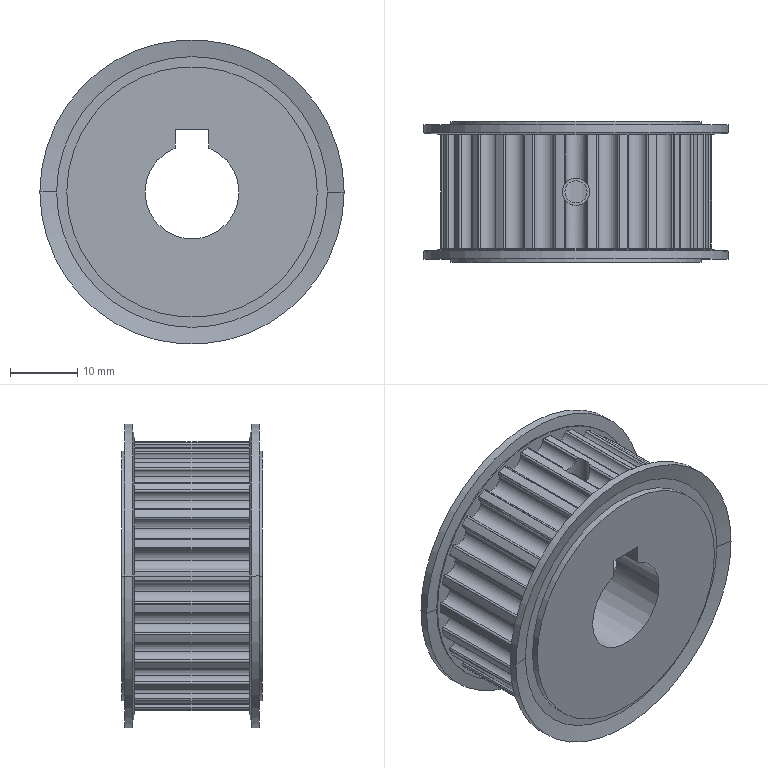Part | STEP file | 1 solid | 237 faces | box 45.32 x 21 x 45.32 mm | volume 21338 mm3 | cylinder 162 | plane 67 | cone 8 | commonest cylinder face diameters 0.488 x72 3 x40 40.24 x27 3.3 x4 4.1 x4 37.32 x4